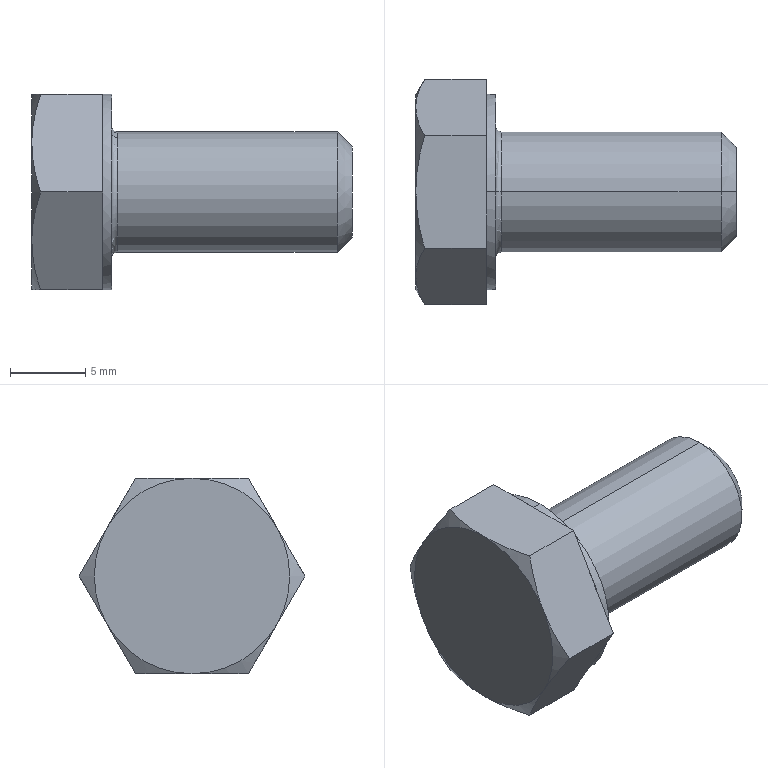Part | SolidWorks | features BaseBody 1 | 1 solid | 29 faces | box 21.3 x 15.011 x 13 mm | volume 1559 mm3 | plane 15 | cone 8 | cylinder 4 | torus 2 | commonest cylinder face diameters 8 x2 13 x2
STEP:
#1=CARTESIAN_POINT('',(5.7,0.,4.));
#2=VERTEX_POINT('',#1);
#3=CARTESIAN_POINT('',(5.3,0.,4.4));
#4=VERTEX_POINT('',#3);
#5=CARTESIAN_POINT('',(5.7,0.,4.4));
#6=DIRECTION('',(0.,1.,0.));
#7=DIRECTION('',(0.,0.,1.));
#8=AXIS2_PLACEMENT_3D('',#5,#6,#7);
#9=CIRCLE('',#8,0.4);
#10=EDGE_CURVE('',#2,#4,#9,.T.);
#11=ORIENTED_EDGE('',*,*,#10,.F.);
#12=CARTESIAN_POINT('',(5.7,0.,-4.));
#13=VERTEX_POINT('',#12);
#14=CARTESIAN_POINT('',(5.7,0.,0.));
#15=DIRECTION('',(1.,0.,0.));
#16=DIRECTION('',(0.,0.,-1.));
#17=AXIS2_PLACEMENT_3D('',#14,#15,#16);
#18=CIRCLE('',#17,4.);
#19=EDGE_CURVE('',#13,#2,#18,.T.);
#20=ORIENTED_EDGE('',*,*,#19,.F.);
#21=CARTESIAN_POINT('',(5.3,0.,-4.4));
#22=VERTEX_POINT('',#21);
#23=CARTESIAN_POINT('',(5.7,0.,-4.4));
#24=DIRECTION('',(0.,-1.,0.));
#25=DIRECTION('',(0.,0.,-1.));
#26=AXIS2_PLACEMENT_3D('',#23,#24,#25);
#27=CIRCLE('',#26,0.4);
#28=EDGE_CURVE('',#13,#22,#27,.T.);
#29=ORIENTED_EDGE('',*,*,#28,.T.);
#30=CARTESIAN_POINT('',(5.3,0.,0.));
#31=DIRECTION('',(-1.,0.,0.));
#32=DIRECTION('',(0.,0.,-1.));
#33=AXIS2_PLACEMENT_3D('',#30,#31,#32);
#34=CIRCLE('',#33,4.4);
#35=EDGE_CURVE('',#4,#22,#34,.T.);
#36=ORIENTED_EDGE('',*,*,#35,.F.);
#37=EDGE_LOOP('',(#11,#20,#29,#36));
#38=FACE_OUTER_BOUND('',#37,.T.);
#39=CARTESIAN_POINT('',(5.7,0.,0.));
#40=DIRECTION('',(1.,0.,0.));
#41=DIRECTION('',(0.,0.,-1.));
#42=AXIS2_PLACEMENT_3D('',#39,#40,#41);
#43=TOROIDAL_SURFACE('',#42,4.4,0.4);
#44=ADVANCED_FACE('',(#38),#43,.F.);
#45=CARTESIAN_POINT('',(21.3,0.,-3.));
#46=VERTEX_POINT('',#45);
#47=CARTESIAN_POINT('',(20.3,0.,-4.));
#48=VERTEX_POINT('',#47);
#49=CARTESIAN_POINT('',(20.3,0.,-4.));
#50=DIRECTION('',(-0.7071,0.,-0.7071));
#51=VECTOR('',#50,1000.);
#52=LINE('',#49,#51);
#53=EDGE_CURVE('',#46,#48,#52,.T.);
#54=ORIENTED_EDGE('',*,*,#53,.F.);
#55=CARTESIAN_POINT('',(21.3,0.,3.));
#56=VERTEX_POINT('',#55);
#57=CARTESIAN_POINT('',(21.3,0.,0.));
#58=DIRECTION('',(1.,0.,0.));
#59=DIRECTION('',(0.,0.,1.));
#60=AXIS2_PLACEMENT_3D('',#57,#58,#59);
#61=CIRCLE('',#60,3.);
#62=EDGE_CURVE('',#56,#46,#61,.T.);
#63=ORIENTED_EDGE('',*,*,#62,.F.);
#64=CARTESIAN_POINT('',(20.3,0.,4.));
#65=VERTEX_POINT('',#64);
#66=CARTESIAN_POINT('',(20.3,0.,4.));
#67=DIRECTION('',(-0.7071,0.,0.7071));
#68=VECTOR('',#67,1000.);
#69=LINE('',#66,#68);
#70=EDGE_CURVE('',#56,#65,#69,.T.);
#71=ORIENTED_EDGE('',*,*,#70,.T.);
#72=CARTESIAN_POINT('',(20.3,0.,0.));
#73=DIRECTION('',(-1.,0.,0.));
#74=DIRECTION('',(0.,0.,1.));
#75=AXIS2_PLACEMENT_3D('',#72,#73,#74);
#76=CIRCLE('',#75,4.);
#77=EDGE_CURVE('',#48,#65,#76,.T.);
#78=ORIENTED_EDGE('',*,*,#77,.F.);
#79=EDGE_LOOP('',(#54,#63,#71,#78));
#80=FACE_OUTER_BOUND('',#79,.T.);
#81=CARTESIAN_POINT('',(20.3,0.,0.));
#82=DIRECTION('',(-1.,0.,0.));
#83=DIRECTION('',(0.,0.,1.));
#84=AXIS2_PLACEMENT_3D('',#81,#82,#83);
#85=CONICAL_SURFACE('',#84,4.,0.7854);
#86=ADVANCED_FACE('',(#80),#85,.T.);
#87=CARTESIAN_POINT('',(5.3,0.,0.));
#88=DIRECTION('',(-1.,0.,0.));
#89=DIRECTION('',(0.,0.,-1.));
#90=AXIS2_PLACEMENT_3D('',#87,#88,#89);
#91=CIRCLE('',#90,4.4);
#92=EDGE_CURVE('',#22,#4,#91,.T.);
#93=ORIENTED_EDGE('',*,*,#92,.T.);
#94=ORIENTED_EDGE('',*,*,#35,.T.);
#95=EDGE_LOOP('',(#93,#94));
#96=FACE_BOUND('',#95,.T.);
#97=CARTESIAN_POINT('',(5.3,0.,6.5));
#98=VERTEX_POINT('',#97);
#99=CARTESIAN_POINT('',(5.3,0.,-6.5));
#100=VERTEX_POINT('',#99);
#101=CARTESIAN_POINT('',(5.3,0.,0.));
#102=DIRECTION('',(1.,0.,0.));
#103=DIRECTION('',(0.,0.,-1.));
#104=AXIS2_PLACEMENT_3D('',#101,#102,#103);
#105=CIRCLE('',#104,6.5);
#106=EDGE_CURVE('',#98,#100,#105,.T.);
#107=ORIENTED_EDGE('',*,*,#106,.T.);
#108=CARTESIAN_POINT('',(5.3,0.,0.));
#109=DIRECTION('',(1.,0.,0.));
#110=DIRECTION('',(0.,0.,-1.));
#111=AXIS2_PLACEMENT_3D('',#108,#109,#110);
#112=CIRCLE('',#111,6.5);
#113=EDGE_CURVE('',#100,#98,#112,.T.);
#114=ORIENTED_EDGE('',*,*,#113,.T.);
#115=EDGE_LOOP('',(#107,#114));
#116=FACE_OUTER_BOUND('',#115,.T.);
#117=CARTESIAN_POINT('',(5.3,7.506,0.));
#118=DIRECTION('',(1.,0.,0.));
#119=DIRECTION('',(0.,1.,0.));
#120=AXIS2_PLACEMENT_3D('',#117,#118,#119);
#121=PLANE('',#120);
#122=ADVANCED_FACE('',(#96,#116),#121,.T.);
#123=CARTESIAN_POINT('',(0.,0.,-4.));
#124=DIRECTION('',(-1.,0.,0.));
#125=VECTOR('',#124,1000.);
#126=LINE('',#123,#125);
#127=EDGE_CURVE('',#48,#13,#126,.T.);
#128=ORIENTED_EDGE('',*,*,#127,.F.);
#129=ORIENTED_EDGE('',*,*,#77,.T.);
#130=CARTESIAN_POINT('',(0.,0.,4.));
#131=DIRECTION('',(-1.,0.,0.));
#132=VECTOR('',#131,1000.);
#133=LINE('',#130,#132);
#134=EDGE_CURVE('',#65,#2,#133,.T.);
#135=ORIENTED_EDGE('',*,*,#134,.T.);
#136=CARTESIAN_POINT('',(5.7,0.,0.));
#137=DIRECTION('',(1.,0.,0.));
#138=DIRECTION('',(0.,0.,-1.));
#139=AXIS2_PLACEMENT_3D('',#136,#137,#138);
#140=CIRCLE('',#139,4.);
#141=EDGE_CURVE('',#2,#13,#140,.T.);
#142=ORIENTED_EDGE('',*,*,#141,.T.);
#143=EDGE_LOOP('',(#128,#129,#135,#142));
#144=FACE_OUTER_BOUND('',#143,.T.);
#145=CARTESIAN_POINT('',(0.,0.,0.));
#146=DIRECTION('',(-1.,0.,0.));
#147=DIRECTION('',(0.,0.,1.));
#148=AXIS2_PLACEMENT_3D('',#145,#146,#147);
#149=CYLINDRICAL_SURFACE('',#148,4.);
#150=ADVANCED_FACE('',(#144),#149,.T.);
#151=ORIENTED_EDGE('',*,*,#62,.T.);
#152=CARTESIAN_POINT('',(21.3,0.,0.));
#153=DIRECTION('',(1.,0.,0.));
#154=DIRECTION('',(0.,0.,1.));
#155=AXIS2_PLACEMENT_3D('',#152,#153,#154);
#156=CIRCLE('',#155,3.);
#157=EDGE_CURVE('',#46,#56,#156,.T.);
#158=ORIENTED_EDGE('',*,*,#157,.T.);
#159=EDGE_LOOP('',(#151,#158));
#160=FACE_OUTER_BOUND('',#159,.T.);
#161=CARTESIAN_POINT('',(21.3,0.,0.));
#162=DIRECTION('',(-1.,0.,0.));
#163=DIRECTION('',(0.,0.,1.));
#164=AXIS2_PLACEMENT_3D('',#161,#162,#163);
#165=PLANE('',#164);
#166=ADVANCED_FACE('',(#160),#165,.F.);
#167=CARTESIAN_POINT('',(4.7,0.,-6.5));
#168=VERTEX_POINT('',#167);
#169=CARTESIAN_POINT('',(0.,0.,-6.5));
#170=DIRECTION('',(-1.,0.,0.));
#171=VECTOR('',#170,1000.);
#172=LINE('',#169,#171);
#173=EDGE_CURVE('',#100,#168,#172,.T.);
#174=ORIENTED_EDGE('',*,*,#173,.F.);
#175=ORIENTED_EDGE('',*,*,#106,.F.);
#176=CARTESIAN_POINT('',(4.7,0.,6.5));
#177=VERTEX_POINT('',#176);
#178=CARTESIAN_POINT('',(0.,0.,6.5));
#179=DIRECTION('',(-1.,0.,0.));
#180=VECTOR('',#179,1000.);
#181=LINE('',#178,#180);
#182=EDGE_CURVE('',#98,#177,#181,.T.);
#183=ORIENTED_EDGE('',*,*,#182,.T.);
#184=CARTESIAN_POINT('',(4.7,-5.629,3.25));
#185=VERTEX_POINT('',#184);
#186=CARTESIAN_POINT('',(4.7,0.,0.));
#187=DIRECTION('',(-1.,0.,0.));
#188=DIRECTION('',(0.,0.,1.));
#189=AXIS2_PLACEMENT_3D('',#186,#187,#188);
#190=CIRCLE('',#189,6.5);
#191=EDGE_CURVE('',#185,#177,#190,.T.);
#192=ORIENTED_EDGE('',*,*,#191,.F.);
#193=CARTESIAN_POINT('',(4.7,-5.629,-3.25));
#194=VERTEX_POINT('',#193);
#195=CARTESIAN_POINT('',(4.7,0.,0.));
#196=DIRECTION('',(-1.,0.,0.));
#197=DIRECTION('',(0.,0.,1.));
#198=AXIS2_PLACEMENT_3D('',#195,#196,#197);
#199=CIRCLE('',#198,6.5);
#200=EDGE_CURVE('',#194,#185,#199,.T.);
#201=ORIENTED_EDGE('',*,*,#200,.F.);
#202=CARTESIAN_POINT('',(4.7,0.,0.));
#203=DIRECTION('',(-1.,0.,0.));
#204=DIRECTION('',(0.,0.,1.));
#205=AXIS2_PLACEMENT_3D('',#202,#203,#204);
#206=CIRCLE('',#205,6.5);
#207=EDGE_CURVE('',#168,#194,#206,.T.);
#208=ORIENTED_EDGE('',*,*,#207,.F.);
#209=EDGE_LOOP('',(#174,#175,#183,#192,#201,#208));
#210=FACE_OUTER_BOUND('',#209,.T.);
#211=CARTESIAN_POINT('',(0.,0.,0.));
#212=DIRECTION('',(-1.,0.,0.));
#213=DIRECTION('',(0.,0.,1.));
#214=AXIS2_PLACEMENT_3D('',#211,#212,#213);
#215=CYLINDRICAL_SURFACE('',#214,6.5);
#216=ADVANCED_FACE('',(#210),#215,.T.);
#217=CARTESIAN_POINT('',(4.7,-3.753,-6.5));
#218=VERTEX_POINT('',#217);
#219=CARTESIAN_POINT('',(4.7,-3.753,-6.5));
#220=DIRECTION('',(0.,0.5,-0.866));
#221=VECTOR('',#220,1000.);
#222=LINE('',#219,#221);
#223=EDGE_CURVE('',#194,#218,#222,.T.);
#224=ORIENTED_EDGE('',*,*,#223,.T.);
#225=CARTESIAN_POINT('',(4.7,3.753,-6.5));
#226=DIRECTION('',(0.,1.,0.));
#227=VECTOR('',#226,1000.);
#228=LINE('',#225,#227);
#229=EDGE_CURVE('',#218,#168,#228,.T.);
#230=ORIENTED_EDGE('',*,*,#229,.T.);
#231=ORIENTED_EDGE('',*,*,#207,.T.);
#232=EDGE_LOOP('',(#224,#230,#231));
#233=FACE_OUTER_BOUND('',#232,.T.);
#234=CARTESIAN_POINT('',(4.7,6.5,0.));
#235=DIRECTION('',(1.,0.,0.));
#236=DIRECTION('',(0.,1.,0.));
#237=AXIS2_PLACEMENT_3D('',#234,#235,#236);
#238=PLANE('',#237);
#239=ADVANCED_FACE('',(#233),#238,.T.);
#240=CARTESIAN_POINT('',(4.7,-7.506,0.));
#241=VERTEX_POINT('',#240);
#242=CARTESIAN_POINT('',(4.7,-7.506,0.));
#243=DIRECTION('',(0.,-0.5,-0.866));
#244=VECTOR('',#243,1000.);
#245=LINE('',#242,#244);
#246=EDGE_CURVE('',#185,#241,#245,.T.);
#247=ORIENTED_EDGE('',*,*,#246,.T.);
#248=CARTESIAN_POINT('',(4.7,-3.753,-6.5));
#249=DIRECTION('',(0.,0.5,-0.866));
#250=VECTOR('',#249,1000.);
#251=LINE('',#248,#250);
#252=EDGE_CURVE('',#241,#194,#251,.T.);
#253=ORIENTED_EDGE('',*,*,#252,.T.);
#254=ORIENTED_EDGE('',*,*,#200,.T.);
#255=EDGE_LOOP('',(#247,#253,#254));
#256=FACE_OUTER_BOUND('',#255,.T.);
#257=CARTESIAN_POINT('',(4.7,6.5,0.));
#258=DIRECTION('',(1.,0.,0.));
#259=DIRECTION('',(0.,1.,0.));
#260=AXIS2_PLACEMENT_3D('',#257,#258,#259);
#261=PLANE('',#260);
#262=ADVANCED_FACE('',(#256),#261,.T.);
#263=CARTESIAN_POINT('',(4.7,-3.753,6.5));
#264=VERTEX_POINT('',#263);
#265=CARTESIAN_POINT('',(4.7,3.753,6.5));
#266=DIRECTION('',(0.,-1.,0.));
#267=VECTOR('',#266,1000.);
#268=LINE('',#265,#267);
#269=EDGE_CURVE('',#177,#264,#268,.T.);
#270=ORIENTED_EDGE('',*,*,#269,.T.);
#271=CARTESIAN_POINT('',(4.7,-7.506,0.));
#272=DIRECTION('',(0.,-0.5,-0.866));
#273=VECTOR('',#272,1000.);
#274=LINE('',#271,#273);
#275=EDGE_CURVE('',#264,#185,#274,.T.);
#276=ORIENTED_EDGE('',*,*,#275,.T.);
#277=ORIENTED_EDGE('',*,*,#191,.T.);
#278=EDGE_LOOP('',(#270,#276,#277));
#279=FACE_OUTER_BOUND('',#278,.T.);
#280=CARTESIAN_POINT('',(4.7,6.5,0.));
#281=DIRECTION('',(1.,0.,0.));
#282=DIRECTION('',(0.,1.,0.));
#283=AXIS2_PLACEMENT_3D('',#280,#281,#282);
#284=PLANE('',#283);
#285=ADVANCED_FACE('',(#279),#284,.T.);
#286=CARTESIAN_POINT('',(4.7,5.629,3.25));
#287=VERTEX_POINT('',#286);
#288=CARTESIAN_POINT('',(4.7,3.753,6.5));
#289=VERTEX_POINT('',#288);
#290=CARTESIAN_POINT('',(4.7,7.506,0.));
#291=DIRECTION('',(0.,-0.5,0.866));
#292=VECTOR('',#291,1000.);
#293=LINE('',#290,#292);
#294=EDGE_CURVE('',#287,#289,#293,.T.);
#295=ORIENTED_EDGE('',*,*,#294,.T.);
#296=CARTESIAN_POINT('',(4.7,3.753,6.5));
#297=DIRECTION('',(0.,-1.,0.));
#298=VECTOR('',#297,1000.);
#299=LINE('',#296,#298);
#300=EDGE_CURVE('',#289,#177,#299,.T.);
#301=ORIENTED_EDGE('',*,*,#300,.T.);
#302=CARTESIAN_POINT('',(4.7,0.,0.));
#303=DIRECTION('',(-1.,0.,0.));
#304=DIRECTION('',(0.,0.,1.));
#305=AXIS2_PLACEMENT_3D('',#302,#303,#304);
#306=CIRCLE('',#305,6.5);
#307=EDGE_CURVE('',#177,#287,#306,.T.);
#308=ORIENTED_EDGE('',*,*,#307,.T.);
#309=EDGE_LOOP('',(#295,#301,#308));
#310=FACE_OUTER_BOUND('',#309,.T.);
#311=CARTESIAN_POINT('',(4.7,6.5,0.));
#312=DIRECTION('',(1.,0.,0.));
#313=DIRECTION('',(0.,1.,0.));
#314=AXIS2_PLACEMENT_3D('',#311,#312,#313);
#315=PLANE('',#314);
#316=ADVANCED_FACE('',(#310),#315,.T.);
#317=CARTESIAN_POINT('',(4.7,5.629,-3.25));
#318=VERTEX_POINT('',#317);
#319=CARTESIAN_POINT('',(4.7,7.506,0.));
#320=VERTEX_POINT('',#319);
#321=CARTESIAN_POINT('',(4.7,3.753,-6.5));
#322=DIRECTION('',(0.,0.5,0.866));
#323=VECTOR('',#322,1000.);
#324=LINE('',#321,#323);
#325=EDGE_CURVE('',#318,#320,#324,.T.);
#326=ORIENTED_EDGE('',*,*,#325,.T.);
#327=CARTESIAN_POINT('',(4.7,7.506,0.));
#328=DIRECTION('',(0.,-0.5,0.866));
#329=VECTOR('',#328,1000.);
#330=LINE('',#327,#329);
#331=EDGE_CURVE('',#320,#287,#330,.T.);
#332=ORIENTED_EDGE('',*,*,#331,.T.);
#333=CARTESIAN_POINT('',(4.7,0.,0.));
#334=DIRECTION('',(-1.,0.,0.));
#335=DIRECTION('',(0.,0.,1.));
#336=AXIS2_PLACEMENT_3D('',#333,#334,#335);
#337=CIRCLE('',#336,6.5);
#338=EDGE_CURVE('',#287,#318,#337,.T.);
#339=ORIENTED_EDGE('',*,*,#338,.T.);
#340=EDGE_LOOP('',(#326,#332,#339));
#341=FACE_OUTER_BOUND('',#340,.T.);
#342=CARTESIAN_POINT('',(4.7,6.5,0.));
#343=DIRECTION('',(1.,0.,0.));
#344=DIRECTION('',(0.,1.,0.));
#345=AXIS2_PLACEMENT_3D('',#342,#343,#344);
#346=PLANE('',#345);
#347=ADVANCED_FACE('',(#341),#346,.T.);
#348=CARTESIAN_POINT('',(4.7,3.753,-6.5));
#349=VERTEX_POINT('',#348);
#350=CARTESIAN_POINT('',(4.7,3.753,-6.5));
#351=DIRECTION('',(0.,0.5,0.866));
#352=VECTOR('',#351,1000.);
#353=LINE('',#350,#352);
#354=EDGE_CURVE('',#349,#318,#353,.T.);
#355=ORIENTED_EDGE('',*,*,#354,.T.);
#356=CARTESIAN_POINT('',(4.7,0.,0.));
#357=DIRECTION('',(-1.,0.,0.));
#358=DIRECTION('',(0.,0.,1.));
#359=AXIS2_PLACEMENT_3D('',#356,#357,#358);
#360=CIRCLE('',#359,6.5);
#361=EDGE_CURVE('',#318,#168,#360,.T.);
#362=ORIENTED_EDGE('',*,*,#361,.T.);
#363=CARTESIAN_POINT('',(4.7,3.753,-6.5));
#364=DIRECTION('',(0.,1.,0.));
#365=VECTOR('',#364,1000.);
#366=LINE('',#363,#365);
#367=EDGE_CURVE('',#168,#349,#366,.T.);
#368=ORIENTED_EDGE('',*,*,#367,.T.);
#369=EDGE_LOOP('',(#355,#362,#368));
#370=FACE_OUTER_BOUND('',#369,.T.);
#371=CARTESIAN_POINT('',(4.7,6.5,0.));
#372=DIRECTION('',(1.,0.,0.));
#373=DIRECTION('',(0.,1.,0.));
#374=AXIS2_PLACEMENT_3D('',#371,#372,#373);
#375=PLANE('',#374);
#376=ADVANCED_FACE('',(#370),#375,.T.);
#377=CARTESIAN_POINT('',(0.,0.,-6.5));
#378=VERTEX_POINT('',#377);
#379=CARTESIAN_POINT('',(0.,5.629,-3.25));
#380=VERTEX_POINT('',#379);
#381=CARTESIAN_POINT('',(0.,0.,0.));
#382=DIRECTION('',(1.,0.,0.));
#383=DIRECTION('',(0.,0.,-1.));
#384=AXIS2_PLACEMENT_3D('',#381,#382,#383);
#385=CIRCLE('',#384,6.5);
#386=EDGE_CURVE('',#378,#380,#385,.T.);
#387=ORIENTED_EDGE('',*,*,#386,.F.);
#388=CARTESIAN_POINT('',(0.,-5.629,-3.25));
#389=VERTEX_POINT('',#388);
#390=CARTESIAN_POINT('',(0.,0.,0.));
#391=DIRECTION('',(1.,0.,0.));
#392=DIRECTION('',(0.,0.,-1.));
#393=AXIS2_PLACEMENT_3D('',#390,#391,#392);
#394=CIRCLE('',#393,6.5);
#395=EDGE_CURVE('',#389,#378,#394,.T.);
#396=ORIENTED_EDGE('',*,*,#395,.F.);
#397=CARTESIAN_POINT('',(0.,-5.629,3.25));
#398=VERTEX_POINT('',#397);
#399=CARTESIAN_POINT('',(0.,0.,0.));
#400=DIRECTION('',(1.,0.,0.));
#401=DIRECTION('',(0.,0.,-1.));
#402=AXIS2_PLACEMENT_3D('',#399,#400,#401);
#403=CIRCLE('',#402,6.5);
#404=EDGE_CURVE('',#398,#389,#403,.T.);
#405=ORIENTED_EDGE('',*,*,#404,.F.);
#406=CARTESIAN_POINT('',(0.,0.,6.5));
#407=VERTEX_POINT('',#406);
#408=CARTESIAN_POINT('',(0.,0.,0.));
#409=DIRECTION('',(1.,0.,0.));
#410=DIRECTION('',(0.,0.,-1.));
#411=AXIS2_PLACEMENT_3D('',#408,#409,#410);
#412=CIRCLE('',#411,6.5);
#413=EDGE_CURVE('',#407,#398,#412,.T.);
#414=ORIENTED_EDGE('',*,*,#413,.F.);
#415=CARTESIAN_POINT('',(0.,5.629,3.25));
#416=VERTEX_POINT('',#415);
#417=CARTESIAN_POINT('',(0.,0.,0.));
#418=DIRECTION('',(-1.,0.,0.));
#419=DIRECTION('',(0.,0.,1.));
#420=AXIS2_PLACEMENT_3D('',#417,#418,#419);
#421=CIRCLE('',#420,6.5);
#422=EDGE_CURVE('',#407,#416,#421,.T.);
#423=ORIENTED_EDGE('',*,*,#422,.T.);
#424=CARTESIAN_POINT('',(0.,0.,0.));
#425=DIRECTION('',(1.,0.,0.));
#426=DIRECTION('',(0.,0.,-1.));
#427=AXIS2_PLACEMENT_3D('',#424,#425,#426);
#428=CIRCLE('',#427,6.5);
#429=EDGE_CURVE('',#380,#416,#428,.T.);
#430=ORIENTED_EDGE('',*,*,#429,.F.);
#431=EDGE_LOOP('',(#387,#396,#405,#414,#423,#430));
#432=FACE_OUTER_BOUND('',#431,.T.);
#433=CARTESIAN_POINT('',(0.,7.506,0.));
#434=DIRECTION('',(1.,0.,0.));
#435=DIRECTION('',(0.,1.,0.));
#436=AXIS2_PLACEMENT_3D('',#433,#434,#435);
#437=PLANE('',#436);
#438=ADVANCED_FACE('',(#432),#437,.F.);
#439=CARTESIAN_POINT('',(0.5806,3.753,-6.5));
#440=VERTEX_POINT('',#439);
#441=CARTESIAN_POINT('',(0.,5.629,-3.25));
#442=CARTESIAN_POINT('',(0.,5.549,-3.388));
#443=CARTESIAN_POINT('',(0.003356,5.47,-3.525));
#444=CARTESIAN_POINT('',(0.01342,5.351,-3.732));
#445=CARTESIAN_POINT('',(0.01762,5.311,-3.801));
#446=CARTESIAN_POINT('',(0.02769,5.232,-3.939));
#447=CARTESIAN_POINT('',(0.0337,5.191,-4.009));
#448=CARTESIAN_POINT('',(0.05342,5.073,-4.213));
#449=CARTESIAN_POINT('',(0.0697,4.995,-4.348));
#450=CARTESIAN_POINT('',(0.09881,4.877,-4.552));
#451=CARTESIAN_POINT('',(0.1145,4.818,-4.654));
#452=CARTESIAN_POINT('',(0.132,4.759,-4.757));
#453=CARTESIAN_POINT('',(0.1441,4.72,-4.825));
#454=CARTESIAN_POINT('',(0.1506,4.699,-4.861));
#455=CARTESIAN_POINT('',(0.2548,4.377,-5.419));
#456=CARTESIAN_POINT('',(0.3961,4.072,-5.947));
#457=CARTESIAN_POINT('',(0.5806,3.753,-6.5));
#458=B_SPLINE_CURVE_WITH_KNOTS('',3,(#441,#442,#443,#444,#445,#446,#447,#448,#449,#450,#451,#452,#453,#454,#455,#456,#457),.UNSPECIFIED.,.F.,.F.,(4,2,2,2,2,1,2,2,4),(0.,0.125,0.1875,0.25,0.375,0.4375,0.4688,0.5,1.),.UNSPECIFIED.);
#459=EDGE_CURVE('',#380,#440,#458,.T.);
#460=ORIENTED_EDGE('',*,*,#459,.T.);
#461=CARTESIAN_POINT('',(0.5806,3.753,-6.5));
#462=CARTESIAN_POINT('',(0.4887,3.435,-6.5));
#463=CARTESIAN_POINT('',(0.4075,3.123,-6.5));
#464=CARTESIAN_POINT('',(0.3018,2.663,-6.5));
#465=CARTESIAN_POINT('',(0.2693,2.511,-6.5));
#466=CARTESIAN_POINT('',(0.2245,2.283,-6.5));
#467=CARTESIAN_POINT('',(0.2031,2.169,-6.5));
#468=CARTESIAN_POINT('',(0.1832,2.056,-6.5));
#469=CARTESIAN_POINT('',(0.1703,1.98,-6.5));
#470=CARTESIAN_POINT('',(0.1643,1.945,-6.5));
#471=CARTESIAN_POINT('',(0.132,1.746,-6.5));
#472=CARTESIAN_POINT('',(0.1093,1.587,-6.5));
#473=CARTESIAN_POINT('',(0.07994,1.351,-6.5));
#474=CARTESIAN_POINT('',(0.07094,1.272,-6.5));
#475=CARTESIAN_POINT('',(0.05452,1.114,-6.5));
#476=CARTESIAN_POINT('',(0.0472,1.036,-6.5));
#477=CARTESIAN_POINT('',(0.01349,0.6346,-6.5));
#478=CARTESIAN_POINT('',(0.,0.3183,-6.5));
#479=CARTESIAN_POINT('',(0.,0.,-6.5));
#480=B_SPLINE_CURVE_WITH_KNOTS('',3,(#461,#462,#463,#464,#465,#466,#467,#468,#469,#470,#471,#472,#473,#474,#475,#476,#477,#478,#479),.UNSPECIFIED.,.F.,.F.,(4,2,2,1,2,2,2,2,2,4),(0.,0.25,0.375,0.4375,0.4687,0.5,0.625,0.6875,0.75,1.),.UNSPECIFIED.);
#481=EDGE_CURVE('',#440,#378,#480,.T.);
#482=ORIENTED_EDGE('',*,*,#481,.T.);
#483=ORIENTED_EDGE('',*,*,#386,.T.);
#484=EDGE_LOOP('',(#460,#482,#483));
#485=FACE_OUTER_BOUND('',#484,.T.);
#486=CARTESIAN_POINT('',(0.,0.,0.));
#487=DIRECTION('',(1.,0.,0.));
#488=DIRECTION('',(0.,0.,-1.));
#489=AXIS2_PLACEMENT_3D('',#486,#487,#488);
#490=CONICAL_SURFACE('',#489,6.5,1.047);
#491=ADVANCED_FACE('',(#485),#490,.T.);
#492=CARTESIAN_POINT('',(0.5806,7.506,0.));
#493=VERTEX_POINT('',#492);
#494=CARTESIAN_POINT('',(0.,5.629,3.25));
#495=CARTESIAN_POINT('',(0.,5.709,3.112));
#496=CARTESIAN_POINT('',(0.003356,5.788,2.974));
#497=CARTESIAN_POINT('',(0.01342,5.907,2.768));
#498=CARTESIAN_POINT('',(0.01762,5.947,2.699));
#499=CARTESIAN_POINT('',(0.02769,6.027,2.561));
#500=CARTESIAN_POINT('',(0.0337,6.067,2.491));
#501=CARTESIAN_POINT('',(0.05342,6.185,2.287));
#502=CARTESIAN_POINT('',(0.0697,6.263,2.152));
#503=CARTESIAN_POINT('',(0.09881,6.381,1.948));
#504=CARTESIAN_POINT('',(0.1145,6.44,1.846));
#505=CARTESIAN_POINT('',(0.132,6.499,1.743));
#506=CARTESIAN_POINT('',(0.1441,6.539,1.675));
#507=CARTESIAN_POINT('',(0.1506,6.559,1.639));
#508=CARTESIAN_POINT('',(0.2548,6.881,1.081));
#509=CARTESIAN_POINT('',(0.3961,7.186,0.5534));
#510=CARTESIAN_POINT('',(0.5806,7.506,0.));
#511=B_SPLINE_CURVE_WITH_KNOTS('',3,(#494,#495,#496,#497,#498,#499,#500,#501,#502,#503,#504,#505,#506,#507,#508,#509,#510),.UNSPECIFIED.,.F.,.F.,(4,2,2,2,2,1,2,2,4),(0.,0.125,0.1875,0.25,0.375,0.4375,0.4688,0.5,1.),.UNSPECIFIED.);
#512=EDGE_CURVE('',#416,#493,#511,.T.);
#513=ORIENTED_EDGE('',*,*,#512,.T.);
#514=CARTESIAN_POINT('',(0.5806,7.506,0.));
#515=CARTESIAN_POINT('',(0.4882,7.346,-0.277));
#516=CARTESIAN_POINT('',(0.4067,7.189,-0.5478));
#517=CARTESIAN_POINT('',(0.3006,6.958,-0.9485));
#518=CARTESIAN_POINT('',(0.268,6.881,-1.081));
#519=CARTESIAN_POINT('',(0.2231,6.767,-1.279));
#520=CARTESIAN_POINT('',(0.2016,6.71,-1.378));
#521=CARTESIAN_POINT('',(0.1817,6.653,-1.477));
#522=CARTESIAN_POINT('',(0.1688,6.615,-1.543));
#523=CARTESIAN_POINT('',(0.1627,6.597,-1.574));
#524=CARTESIAN_POINT('',(0.1307,6.498,-1.745));
#525=CARTESIAN_POINT('',(0.1083,6.419,-1.882));
#526=CARTESIAN_POINT('',(0.07923,6.302,-2.085));
#527=CARTESIAN_POINT('',(0.07033,6.262,-2.153));
#528=CARTESIAN_POINT('',(0.05409,6.184,-2.289));
#529=CARTESIAN_POINT('',(0.04688,6.146,-2.355));
#530=CARTESIAN_POINT('',(0.01339,5.946,-2.701));
#531=CARTESIAN_POINT('',(0.,5.788,-2.975));
#532=CARTESIAN_POINT('',(0.,5.629,-3.25));
#533=B_SPLINE_CURVE_WITH_KNOTS('',3,(#514,#515,#516,#517,#518,#519,#520,#521,#522,#523,#524,#525,#526,#527,#528,#529,#530,#531,#532),.UNSPECIFIED.,.F.,.F.,(4,2,2,1,2,2,2,2,2,4),(0.,0.25,0.375,0.4375,0.4688,0.5,0.625,0.6875,0.75,1.),.UNSPECIFIED.);
#534=EDGE_CURVE('',#493,#380,#533,.T.);
#535=ORIENTED_EDGE('',*,*,#534,.T.);
#536=ORIENTED_EDGE('',*,*,#429,.T.);
#537=EDGE_LOOP('',(#513,#535,#536));
#538=FACE_OUTER_BOUND('',#537,.T.);
#539=CARTESIAN_POINT('',(0.,0.,0.));
#540=DIRECTION('',(1.,0.,0.));
#541=DIRECTION('',(0.,0.,-1.));
#542=AXIS2_PLACEMENT_3D('',#539,#540,#541);
#543=CONICAL_SURFACE('',#542,6.5,1.047);
#544=ADVANCED_FACE('',(#538),#543,.T.);
#545=CARTESIAN_POINT('',(0.5806,3.753,6.5));
#546=VERTEX_POINT('',#545);
#547=CARTESIAN_POINT('',(0.,0.,6.5));
#548=CARTESIAN_POINT('',(0.,0.1591,6.5));
#549=CARTESIAN_POINT('',(0.003371,0.3178,6.5));
#550=CARTESIAN_POINT('',(0.01349,0.5563,6.5));
#551=CARTESIAN_POINT('',(0.0177,0.6359,6.5));
#552=CARTESIAN_POINT('',(0.02781,0.7955,6.5));
#553=CARTESIAN_POINT('',(0.03382,0.8767,6.5));
#554=CARTESIAN_POINT('',(0.05373,1.114,6.5));
#555=CARTESIAN_POINT('',(0.07015,1.272,6.5));
#556=CARTESIAN_POINT('',(0.09949,1.508,6.5));
#557=CARTESIAN_POINT('',(0.1153,1.627,6.5));
#558=CARTESIAN_POINT('',(0.133,1.746,6.5));
#559=CARTESIAN_POINT('',(0.1451,1.825,6.5));
#560=CARTESIAN_POINT('',(0.1517,1.867,6.5));
#561=CARTESIAN_POINT('',(0.2559,2.509,6.5));
#562=CARTESIAN_POINT('',(0.3968,3.116,6.5));
#563=CARTESIAN_POINT('',(0.5806,3.753,6.5));
#564=B_SPLINE_CURVE_WITH_KNOTS('',3,(#547,#548,#549,#550,#551,#552,#553,#554,#555,#556,#557,#558,#559,#560,#561,#562,#563),.UNSPECIFIED.,.F.,.F.,(4,2,2,2,2,1,2,2,4),(0.,0.125,0.1875,0.25,0.375,0.4375,0.4688,0.5,1.),.UNSPECIFIED.);
#565=EDGE_CURVE('',#407,#546,#564,.T.);
#566=ORIENTED_EDGE('',*,*,#565,.T.);
#567=CARTESIAN_POINT('',(0.5806,3.753,6.5));
#568=CARTESIAN_POINT('',(0.4882,3.913,6.223));
#569=CARTESIAN_POINT('',(0.4067,4.069,5.952));
#570=CARTESIAN_POINT('',(0.3006,4.3,5.551));
#571=CARTESIAN_POINT('',(0.268,4.377,5.419));
#572=CARTESIAN_POINT('',(0.2231,4.491,5.221));
#573=CARTESIAN_POINT('',(0.2016,4.548,5.122));
#574=CARTESIAN_POINT('',(0.1817,4.605,5.023));
#575=CARTESIAN_POINT('',(0.1688,4.643,4.957));
#576=CARTESIAN_POINT('',(0.1627,4.662,4.926));
#577=CARTESIAN_POINT('',(0.1307,4.76,4.755));
#578=CARTESIAN_POINT('',(0.1083,4.839,4.618));
#579=CARTESIAN_POINT('',(0.07923,4.957,4.415));
#580=CARTESIAN_POINT('',(0.07033,4.996,4.347));
#581=CARTESIAN_POINT('',(0.05409,5.074,4.211));
#582=CARTESIAN_POINT('',(0.04688,5.113,4.145));
#583=CARTESIAN_POINT('',(0.01339,5.312,3.799));
#584=CARTESIAN_POINT('',(0.,5.47,3.525));
#585=CARTESIAN_POINT('',(0.,5.629,3.25));
#586=B_SPLINE_CURVE_WITH_KNOTS('',3,(#567,#568,#569,#570,#571,#572,#573,#574,#575,#576,#577,#578,#579,#580,#581,#582,#583,#584,#585),.UNSPECIFIED.,.F.,.F.,(4,2,2,1,2,2,2,2,2,4),(0.,0.25,0.375,0.4375,0.4687,0.5,0.625,0.6875,0.75,1.),.UNSPECIFIED.);
#587=EDGE_CURVE('',#546,#416,#586,.T.);
#588=ORIENTED_EDGE('',*,*,#587,.T.);
#589=ORIENTED_EDGE('',*,*,#422,.F.);
#590=EDGE_LOOP('',(#566,#588,#589));
#591=FACE_OUTER_BOUND('',#590,.T.);
#592=CARTESIAN_POINT('',(0.,0.,0.));
#593=DIRECTION('',(1.,0.,0.));
#594=DIRECTION('',(0.,0.,-1.));
#595=AXIS2_PLACEMENT_3D('',#592,#593,#594);
#596=CONICAL_SURFACE('',#595,6.5,1.047);
#597=ADVANCED_FACE('',(#591),#596,.T.);
#598=CARTESIAN_POINT('',(0.5806,-3.753,6.5));
#599=VERTEX_POINT('',#598);
#600=CARTESIAN_POINT('',(0.5806,-3.753,6.5));
#601=CARTESIAN_POINT('',(0.488,-3.432,6.5));
#602=CARTESIAN_POINT('',(0.4063,-3.118,6.5));
#603=CARTESIAN_POINT('',(0.3,-2.655,6.5));
#604=CARTESIAN_POINT('',(0.2673,-2.501,6.5));
#605=CARTESIAN_POINT('',(0.2223,-2.272,6.5));
#606=CARTESIAN_POINT('',(0.2009,-2.157,6.5));
#607=CARTESIAN_POINT('',(0.1809,-2.043,6.5));
#608=CARTESIAN_POINT('',(0.168,-1.967,6.5));
#609=CARTESIAN_POINT('',(0.1619,-1.93,6.5));
#610=CARTESIAN_POINT('',(0.13,-1.733,6.5));
#611=CARTESIAN_POINT('',(0.1076,-1.575,6.5));
#612=CARTESIAN_POINT('',(0.07869,-1.34,6.5));
#613=CARTESIAN_POINT('',(0.06982,-1.262,6.5));
#614=CARTESIAN_POINT('',(0.05364,-1.105,6.5));
#615=CARTESIAN_POINT('',(0.04643,-1.028,6.5));
#616=CARTESIAN_POINT('',(0.01327,-0.6305,6.5));
#617=CARTESIAN_POINT('',(0.,-0.3164,6.5));
#618=CARTESIAN_POINT('',(0.,0.,6.5));
#619=B_SPLINE_CURVE_WITH_KNOTS('',3,(#600,#601,#602,#603,#604,#605,#606,#607,#608,#609,#610,#611,#612,#613,#614,#615,#616,#617,#618),.UNSPECIFIED.,.F.,.F.,(4,2,2,1,2,2,2,2,2,4),(0.,0.25,0.375,0.4375,0.4688,0.5,0.625,0.6875,0.75,1.),.UNSPECIFIED.);
#620=EDGE_CURVE('',#599,#407,#619,.T.);
#621=ORIENTED_EDGE('',*,*,#620,.T.);
#622=ORIENTED_EDGE('',*,*,#413,.T.);
#623=CARTESIAN_POINT('',(0.,-5.629,3.25));
#624=CARTESIAN_POINT('',(0.,-5.549,3.388));
#625=CARTESIAN_POINT('',(0.003356,-5.47,3.525));
#626=CARTESIAN_POINT('',(0.01342,-5.351,3.732));
#627=CARTESIAN_POINT('',(0.01762,-5.311,3.801));
#628=CARTESIAN_POINT('',(0.02769,-5.232,3.939));
#629=CARTESIAN_POINT('',(0.0337,-5.191,4.009));
#630=CARTESIAN_POINT('',(0.05342,-5.073,4.213));
#631=CARTESIAN_POINT('',(0.0697,-4.995,4.348));
#632=CARTESIAN_POINT('',(0.09881,-4.877,4.552));
#633=CARTESIAN_POINT('',(0.1145,-4.818,4.654));
#634=CARTESIAN_POINT('',(0.132,-4.759,4.757));
#635=CARTESIAN_POINT('',(0.1441,-4.72,4.825));
#636=CARTESIAN_POINT('',(0.1506,-4.699,4.861));
#637=CARTESIAN_POINT('',(0.2548,-4.377,5.419));
#638=CARTESIAN_POINT('',(0.3961,-4.072,5.947));
#639=CARTESIAN_POINT('',(0.5806,-3.753,6.5));
#640=B_SPLINE_CURVE_WITH_KNOTS('',3,(#623,#624,#625,#626,#627,#628,#629,#630,#631,#632,#633,#634,#635,#636,#637,#638,#639),.UNSPECIFIED.,.F.,.F.,(4,2,2,2,2,1,2,2,4),(0.,0.125,0.1875,0.25,0.375,0.4375,0.4688,0.5,1.),.UNSPECIFIED.);
#641=EDGE_CURVE('',#398,#599,#640,.T.);
#642=ORIENTED_EDGE('',*,*,#641,.T.);
#643=EDGE_LOOP('',(#621,#622,#642));
#644=FACE_OUTER_BOUND('',#643,.T.);
#645=CARTESIAN_POINT('',(0.,0.,0.));
#646=DIRECTION('',(1.,0.,0.));
#647=DIRECTION('',(0.,0.,-1.));
#648=AXIS2_PLACEMENT_3D('',#645,#646,#647);
#649=CONICAL_SURFACE('',#648,6.5,1.047);
#650=ADVANCED_FACE('',(#644),#649,.T.);
#651=CARTESIAN_POINT('',(0.5806,-7.506,0.));
#652=VERTEX_POINT('',#651);
#653=CARTESIAN_POINT('',(0.5806,-7.506,0.));
#654=CARTESIAN_POINT('',(0.4882,-7.346,0.277));
#655=CARTESIAN_POINT('',(0.4067,-7.189,0.5478));
#656=CARTESIAN_POINT('',(0.3006,-6.958,0.9485));
#657=CARTESIAN_POINT('',(0.268,-6.881,1.081));
#658=CARTESIAN_POINT('',(0.2231,-6.767,1.279));
#659=CARTESIAN_POINT('',(0.2016,-6.71,1.378));
#660=CARTESIAN_POINT('',(0.1817,-6.653,1.477));
#661=CARTESIAN_POINT('',(0.1688,-6.615,1.543));
#662=CARTESIAN_POINT('',(0.1627,-6.597,1.574));
#663=CARTESIAN_POINT('',(0.1307,-6.498,1.745));
#664=CARTESIAN_POINT('',(0.1083,-6.419,1.882));
#665=CARTESIAN_POINT('',(0.07923,-6.302,2.085));
#666=CARTESIAN_POINT('',(0.07033,-6.262,2.153));
#667=CARTESIAN_POINT('',(0.05409,-6.184,2.289));
#668=CARTESIAN_POINT('',(0.04688,-6.146,2.355));
#669=CARTESIAN_POINT('',(0.01339,-5.946,2.701));
#670=CARTESIAN_POINT('',(0.,-5.788,2.975));
#671=CARTESIAN_POINT('',(0.,-5.629,3.25));
#672=B_SPLINE_CURVE_WITH_KNOTS('',3,(#653,#654,#655,#656,#657,#658,#659,#660,#661,#662,#663,#664,#665,#666,#667,#668,#669,#670,#671),.UNSPECIFIED.,.F.,.F.,(4,2,2,1,2,2,2,2,2,4),(0.,0.25,0.375,0.4375,0.4687,0.5,0.625,0.6875,0.75,1.),.UNSPECIFIED.);
#673=EDGE_CURVE('',#652,#398,#672,.T.);
#674=ORIENTED_EDGE('',*,*,#673,.T.);
#675=ORIENTED_EDGE('',*,*,#404,.T.);
#676=CARTESIAN_POINT('',(0.,-5.629,-3.25));
#677=CARTESIAN_POINT('',(0.,-5.709,-3.112));
#678=CARTESIAN_POINT('',(0.003356,-5.788,-2.974));
#679=CARTESIAN_POINT('',(0.01342,-5.907,-2.768));
#680=CARTESIAN_POINT('',(0.01762,-5.947,-2.699));
#681=CARTESIAN_POINT('',(0.02769,-6.027,-2.561));
#682=CARTESIAN_POINT('',(0.0337,-6.067,-2.491));
#683=CARTESIAN_POINT('',(0.05342,-6.185,-2.287));
#684=CARTESIAN_POINT('',(0.0697,-6.263,-2.152));
#685=CARTESIAN_POINT('',(0.09881,-6.381,-1.948));
#686=CARTESIAN_POINT('',(0.1145,-6.44,-1.846));
#687=CARTESIAN_POINT('',(0.132,-6.499,-1.743));
#688=CARTESIAN_POINT('',(0.1441,-6.539,-1.675));
#689=CARTESIAN_POINT('',(0.1506,-6.559,-1.639));
#690=CARTESIAN_POINT('',(0.2548,-6.881,-1.081));
#691=CARTESIAN_POINT('',(0.3961,-7.186,-0.5534));
#692=CARTESIAN_POINT('',(0.5806,-7.506,0.));
#693=B_SPLINE_CURVE_WITH_KNOTS('',3,(#676,#677,#678,#679,#680,#681,#682,#683,#684,#685,#686,#687,#688,#689,#690,#691,#692),.UNSPECIFIED.,.F.,.F.,(4,2,2,2,2,1,2,2,4),(0.,0.125,0.1875,0.25,0.375,0.4375,0.4688,0.5,1.),.UNSPECIFIED.);
#694=EDGE_CURVE('',#389,#652,#693,.T.);
#695=ORIENTED_EDGE('',*,*,#694,.T.);
#696=EDGE_LOOP('',(#674,#675,#695));
#697=FACE_OUTER_BOUND('',#696,.T.);
#698=CARTESIAN_POINT('',(0.,0.,0.));
#699=DIRECTION('',(1.,0.,0.));
#700=DIRECTION('',(0.,0.,-1.));
#701=AXIS2_PLACEMENT_3D('',#698,#699,#700);
#702=CONICAL_SURFACE('',#701,6.5,1.047);
#703=ADVANCED_FACE('',(#697),#702,.T.);
#704=CARTESIAN_POINT('',(0.5806,-3.753,-6.5));
#705=VERTEX_POINT('',#704);
#706=CARTESIAN_POINT('',(0.5806,-3.753,-6.5));
#707=CARTESIAN_POINT('',(0.4882,-3.913,-6.223));
#708=CARTESIAN_POINT('',(0.4067,-4.069,-5.952));
#709=CARTESIAN_POINT('',(0.3006,-4.3,-5.551));
#710=CARTESIAN_POINT('',(0.268,-4.377,-5.419));
#711=CARTESIAN_POINT('',(0.2231,-4.491,-5.221));
#712=CARTESIAN_POINT('',(0.2016,-4.548,-5.122));
#713=CARTESIAN_POINT('',(0.1817,-4.605,-5.023));
#714=CARTESIAN_POINT('',(0.1688,-4.643,-4.957));
#715=CARTESIAN_POINT('',(0.1627,-4.662,-4.926));
#716=CARTESIAN_POINT('',(0.1307,-4.76,-4.755));
#717=CARTESIAN_POINT('',(0.1083,-4.839,-4.618));
#718=CARTESIAN_POINT('',(0.07923,-4.957,-4.415));
#719=CARTESIAN_POINT('',(0.07033,-4.996,-4.347));
#720=CARTESIAN_POINT('',(0.05409,-5.074,-4.211));
#721=CARTESIAN_POINT('',(0.04688,-5.113,-4.145));
#722=CARTESIAN_POINT('',(0.01339,-5.312,-3.799));
#723=CARTESIAN_POINT('',(0.,-5.47,-3.525));
#724=CARTESIAN_POINT('',(0.,-5.629,-3.25));
#725=B_SPLINE_CURVE_WITH_KNOTS('',3,(#706,#707,#708,#709,#710,#711,#712,#713,#714,#715,#716,#717,#718,#719,#720,#721,#722,#723,#724),.UNSPECIFIED.,.F.,.F.,(4,2,2,1,2,2,2,2,2,4),(0.,0.25,0.375,0.4375,0.4688,0.5,0.625,0.6875,0.75,1.),.UNSPECIFIED.);
#726=EDGE_CURVE('',#705,#389,#725,.T.);
#727=ORIENTED_EDGE('',*,*,#726,.T.);
#728=ORIENTED_EDGE('',*,*,#395,.T.);
#729=CARTESIAN_POINT('',(0.,0.,-6.5));
#730=CARTESIAN_POINT('',(0.,-0.1582,-6.5));
#731=CARTESIAN_POINT('',(0.003316,-0.3158,-6.5));
#732=CARTESIAN_POINT('',(0.01327,-0.5526,-6.5));
#733=CARTESIAN_POINT('',(0.01741,-0.6315,-6.5));
#734=CARTESIAN_POINT('',(0.02736,-0.7898,-6.5));
#735=CARTESIAN_POINT('',(0.03326,-0.8703,-6.5));
#736=CARTESIAN_POINT('',(0.05286,-1.105,-6.5));
#737=CARTESIAN_POINT('',(0.06904,-1.262,-6.5));
#738=CARTESIAN_POINT('',(0.09798,-1.497,-6.5));
#739=CARTESIAN_POINT('',(0.1136,-1.615,-6.5));
#740=CARTESIAN_POINT('',(0.131,-1.733,-6.5));
#741=CARTESIAN_POINT('',(0.143,-1.812,-6.5));
#742=CARTESIAN_POINT('',(0.1494,-1.853,-6.5));
#743=CARTESIAN_POINT('',(0.2537,-2.499,-6.5));
#744=CARTESIAN_POINT('',(0.3954,-3.111,-6.5));
#745=CARTESIAN_POINT('',(0.5806,-3.753,-6.5));
#746=B_SPLINE_CURVE_WITH_KNOTS('',3,(#729,#730,#731,#732,#733,#734,#735,#736,#737,#738,#739,#740,#741,#742,#743,#744,#745),.UNSPECIFIED.,.F.,.F.,(4,2,2,2,2,1,2,2,4),(0.,0.125,0.1875,0.25,0.375,0.4375,0.4687,0.5,1.),.UNSPECIFIED.);
#747=EDGE_CURVE('',#378,#705,#746,.T.);
#748=ORIENTED_EDGE('',*,*,#747,.T.);
#749=EDGE_LOOP('',(#727,#728,#748));
#750=FACE_OUTER_BOUND('',#749,.T.);
#751=CARTESIAN_POINT('',(0.,0.,0.));
#752=DIRECTION('',(1.,0.,0.));
#753=DIRECTION('',(0.,0.,-1.));
#754=AXIS2_PLACEMENT_3D('',#751,#752,#753);
#755=CONICAL_SURFACE('',#754,6.5,1.047);
#756=ADVANCED_FACE('',(#750),#755,.T.);
#757=ORIENTED_EDGE('',*,*,#229,.F.);
#758=CARTESIAN_POINT('',(5.3,-3.753,-6.5));
#759=DIRECTION('',(-1.,0.,0.));
#760=VECTOR('',#759,1000.);
#761=LINE('',#758,#760);
#762=EDGE_CURVE('',#218,#705,#761,.T.);
#763=ORIENTED_EDGE('',*,*,#762,.T.);
#764=ORIENTED_EDGE('',*,*,#747,.F.);
#765=ORIENTED_EDGE('',*,*,#481,.F.);
#766=CARTESIAN_POINT('',(5.3,3.753,-6.5));
#767=DIRECTION('',(-1.,0.,0.));
#768=VECTOR('',#767,1000.);
#769=LINE('',#766,#768);
#770=EDGE_CURVE('',#349,#440,#769,.T.);
#771=ORIENTED_EDGE('',*,*,#770,.F.);
#772=ORIENTED_EDGE('',*,*,#367,.F.);
#773=EDGE_LOOP('',(#757,#763,#764,#765,#771,#772));
#774=FACE_OUTER_BOUND('',#773,.T.);
#775=CARTESIAN_POINT('',(5.3,3.753,-6.5));
#776=DIRECTION('',(0.,0.,1.));
#777=DIRECTION('',(0.,-1.,0.));
#778=AXIS2_PLACEMENT_3D('',#775,#776,#777);
#779=PLANE('',#778);
#780=ADVANCED_FACE('',(#774),#779,.F.);
#781=ORIENTED_EDGE('',*,*,#252,.F.);
#782=CARTESIAN_POINT('',(5.3,-7.506,0.));
#783=DIRECTION('',(-1.,0.,0.));
#784=VECTOR('',#783,1000.);
#785=LINE('',#782,#784);
#786=EDGE_CURVE('',#241,#652,#785,.T.);
#787=ORIENTED_EDGE('',*,*,#786,.T.);
#788=ORIENTED_EDGE('',*,*,#694,.F.);
#789=ORIENTED_EDGE('',*,*,#726,.F.);
#790=ORIENTED_EDGE('',*,*,#762,.F.);
#791=ORIENTED_EDGE('',*,*,#223,.F.);
#792=EDGE_LOOP('',(#781,#787,#788,#789,#790,#791));
#793=FACE_OUTER_BOUND('',#792,.T.);
#794=CARTESIAN_POINT('',(5.3,-3.753,-6.5));
#795=DIRECTION('',(0.,0.866,0.5));
#796=DIRECTION('',(1.,0.,0.));
#797=AXIS2_PLACEMENT_3D('',#794,#795,#796);
#798=PLANE('',#797);
#799=ADVANCED_FACE('',(#793),#798,.F.);
#800=ORIENTED_EDGE('',*,*,#275,.F.);
#801=CARTESIAN_POINT('',(5.3,-3.753,6.5));
#802=DIRECTION('',(-1.,0.,0.));
#803=VECTOR('',#802,1000.);
#804=LINE('',#801,#803);
#805=EDGE_CURVE('',#264,#599,#804,.T.);
#806=ORIENTED_EDGE('',*,*,#805,.T.);
#807=ORIENTED_EDGE('',*,*,#641,.F.);
#808=ORIENTED_EDGE('',*,*,#673,.F.);
#809=ORIENTED_EDGE('',*,*,#786,.F.);
#810=ORIENTED_EDGE('',*,*,#246,.F.);
#811=EDGE_LOOP('',(#800,#806,#807,#808,#809,#810));
#812=FACE_OUTER_BOUND('',#811,.T.);
#813=CARTESIAN_POINT('',(5.3,-7.506,0.));
#814=DIRECTION('',(0.,0.866,-0.5));
#815=DIRECTION('',(-1.,0.,0.));
#816=AXIS2_PLACEMENT_3D('',#813,#814,#815);
#817=PLANE('',#816);
#818=ADVANCED_FACE('',(#812),#817,.F.);
#819=ORIENTED_EDGE('',*,*,#300,.F.);
#820=CARTESIAN_POINT('',(5.3,3.753,6.5));
#821=DIRECTION('',(-1.,0.,0.));
#822=VECTOR('',#821,1000.);
#823=LINE('',#820,#822);
#824=EDGE_CURVE('',#289,#546,#823,.T.);
#825=ORIENTED_EDGE('',*,*,#824,.T.);
#826=ORIENTED_EDGE('',*,*,#565,.F.);
#827=ORIENTED_EDGE('',*,*,#620,.F.);
#828=ORIENTED_EDGE('',*,*,#805,.F.);
#829=ORIENTED_EDGE('',*,*,#269,.F.);
#830=EDGE_LOOP('',(#819,#825,#826,#827,#828,#829));
#831=FACE_OUTER_BOUND('',#830,.T.);
#832=CARTESIAN_POINT('',(5.3,3.753,6.5));
#833=DIRECTION('',(0.,0.,-1.));
#834=DIRECTION('',(0.,-1.,0.));
#835=AXIS2_PLACEMENT_3D('',#832,#833,#834);
#836=PLANE('',#835);
#837=ADVANCED_FACE('',(#831),#836,.F.);
#838=ORIENTED_EDGE('',*,*,#331,.F.);
#839=CARTESIAN_POINT('',(5.3,7.506,0.));
#840=DIRECTION('',(-1.,0.,0.));
#841=VECTOR('',#840,1000.);
#842=LINE('',#839,#841);
#843=EDGE_CURVE('',#320,#493,#842,.T.);
#844=ORIENTED_EDGE('',*,*,#843,.T.);
#845=ORIENTED_EDGE('',*,*,#512,.F.);
#846=ORIENTED_EDGE('',*,*,#587,.F.);
#847=ORIENTED_EDGE('',*,*,#824,.F.);
#848=ORIENTED_EDGE('',*,*,#294,.F.);
#849=EDGE_LOOP('',(#838,#844,#845,#846,#847,#848));
#850=FACE_OUTER_BOUND('',#849,.T.);
#851=CARTESIAN_POINT('',(5.3,7.506,0.));
#852=DIRECTION('',(0.,-0.866,-0.5));
#853=DIRECTION('',(0.,0.5,-0.866));
#854=AXIS2_PLACEMENT_3D('',#851,#852,#853);
#855=PLANE('',#854);
#856=ADVANCED_FACE('',(#850),#855,.F.);
#857=ORIENTED_EDGE('',*,*,#354,.F.);
#858=ORIENTED_EDGE('',*,*,#770,.T.);
#859=ORIENTED_EDGE('',*,*,#459,.F.);
#860=ORIENTED_EDGE('',*,*,#534,.F.);
#861=ORIENTED_EDGE('',*,*,#843,.F.);
#862=ORIENTED_EDGE('',*,*,#325,.F.);
#863=EDGE_LOOP('',(#857,#858,#859,#860,#861,#862));
#864=FACE_OUTER_BOUND('',#863,.T.);
#865=CARTESIAN_POINT('',(5.3,3.753,-6.5));
#866=DIRECTION('',(0.,-0.866,0.5));
#867=DIRECTION('',(-1.,0.,0.));
#868=AXIS2_PLACEMENT_3D('',#865,#866,#867);
#869=PLANE('',#868);
#870=ADVANCED_FACE('',(#864),#869,.F.);
#871=ORIENTED_EDGE('',*,*,#113,.F.);
#872=ORIENTED_EDGE('',*,*,#173,.T.);
#873=ORIENTED_EDGE('',*,*,#361,.F.);
#874=ORIENTED_EDGE('',*,*,#338,.F.);
#875=ORIENTED_EDGE('',*,*,#307,.F.);
#876=ORIENTED_EDGE('',*,*,#182,.F.);
#877=EDGE_LOOP('',(#871,#872,#873,#874,#875,#876));
#878=FACE_OUTER_BOUND('',#877,.T.);
#879=CARTESIAN_POINT('',(0.,0.,0.));
#880=DIRECTION('',(-1.,0.,0.));
#881=DIRECTION('',(0.,0.,1.));
#882=AXIS2_PLACEMENT_3D('',#879,#880,#881);
#883=CYLINDRICAL_SURFACE('',#882,6.5);
#884=ADVANCED_FACE('',(#878),#883,.T.);
#885=CARTESIAN_POINT('',(20.3,0.,0.));
#886=DIRECTION('',(-1.,0.,0.));
#887=DIRECTION('',(0.,0.,1.));
#888=AXIS2_PLACEMENT_3D('',#885,#886,#887);
#889=CIRCLE('',#888,4.);
#890=EDGE_CURVE('',#65,#48,#889,.T.);
#891=ORIENTED_EDGE('',*,*,#890,.T.);
#892=ORIENTED_EDGE('',*,*,#127,.T.);
#893=ORIENTED_EDGE('',*,*,#19,.T.);
#894=ORIENTED_EDGE('',*,*,#134,.F.);
#895=EDGE_LOOP('',(#891,#892,#893,#894));
#896=FACE_OUTER_BOUND('',#895,.T.);
#897=CARTESIAN_POINT('',(0.,0.,0.));
#898=DIRECTION('',(-1.,0.,0.));
#899=DIRECTION('',(0.,0.,1.));
#900=AXIS2_PLACEMENT_3D('',#897,#898,#899);
#901=CYLINDRICAL_SURFACE('',#900,4.);
#902=ADVANCED_FACE('',(#896),#901,.T.);
#903=ORIENTED_EDGE('',*,*,#157,.F.);
#904=ORIENTED_EDGE('',*,*,#53,.T.);
#905=ORIENTED_EDGE('',*,*,#890,.F.);
#906=ORIENTED_EDGE('',*,*,#70,.F.);
#907=EDGE_LOOP('',(#903,#904,#905,#906));
#908=FACE_OUTER_BOUND('',#907,.T.);
#909=CARTESIAN_POINT('',(20.3,0.,0.));
#910=DIRECTION('',(-1.,0.,0.));
#911=DIRECTION('',(0.,0.,1.));
#912=AXIS2_PLACEMENT_3D('',#909,#910,#911);
#913=CONICAL_SURFACE('',#912,4.,0.7854);
#914=ADVANCED_FACE('',(#908),#913,.T.);
#915=ORIENTED_EDGE('',*,*,#141,.F.);
#916=ORIENTED_EDGE('',*,*,#10,.T.);
#917=ORIENTED_EDGE('',*,*,#92,.F.);
#918=ORIENTED_EDGE('',*,*,#28,.F.);
#919=EDGE_LOOP('',(#915,#916,#917,#918));
#920=FACE_OUTER_BOUND('',#919,.T.);
#921=CARTESIAN_POINT('',(5.7,0.,0.));
#922=DIRECTION('',(1.,0.,0.));
#923=DIRECTION('',(0.,0.,-1.));
#924=AXIS2_PLACEMENT_3D('',#921,#922,#923);
#925=TOROIDAL_SURFACE('',#924,4.4,0.4);
#926=ADVANCED_FACE('',(#920),#925,.F.);
#927=CLOSED_SHELL('',(#44,#86,#122,#150,#166,#216,#239,#262,#285,#316,#347,#376,#438,#491,#544,#597,#650,#703,#756,#780,#799,#818,#837,#856,#870,#884,#902,#914,#926));
#928=MANIFOLD_SOLID_BREP('',#927);
#929=CARTESIAN_POINT('',(0.,0.,0.));
#930=DIRECTION('',(0.,0.,1.));
#931=DIRECTION('',(1.,0.,0.));
#932=AXIS2_PLACEMENT_3D('',#929,#930,#931);
#933=(LENGTH_UNIT()NAMED_UNIT(*)SI_UNIT(.MILLI.,.METRE.));
#934=UNCERTAINTY_MEASURE_WITH_UNIT(LENGTH_MEASURE(0.00001),#933,'','');
#935=(NAMED_UNIT(*)PLANE_ANGLE_UNIT()SI_UNIT($,.RADIAN.));
#936=(NAMED_UNIT(*)SI_UNIT($,.STERADIAN.)SOLID_ANGLE_UNIT());
#937=(GEOMETRIC_REPRESENTATION_CONTEXT(3)GLOBAL_UNCERTAINTY_ASSIGNED_CONTEXT((#934))GLOBAL_UNIT_ASSIGNED_CONTEXT((#933,#935,#936))REPRESENTATION_CONTEXT('',''));
#938=ADVANCED_BREP_SHAPE_REPRESENTATION('',(#928,#932),#937);